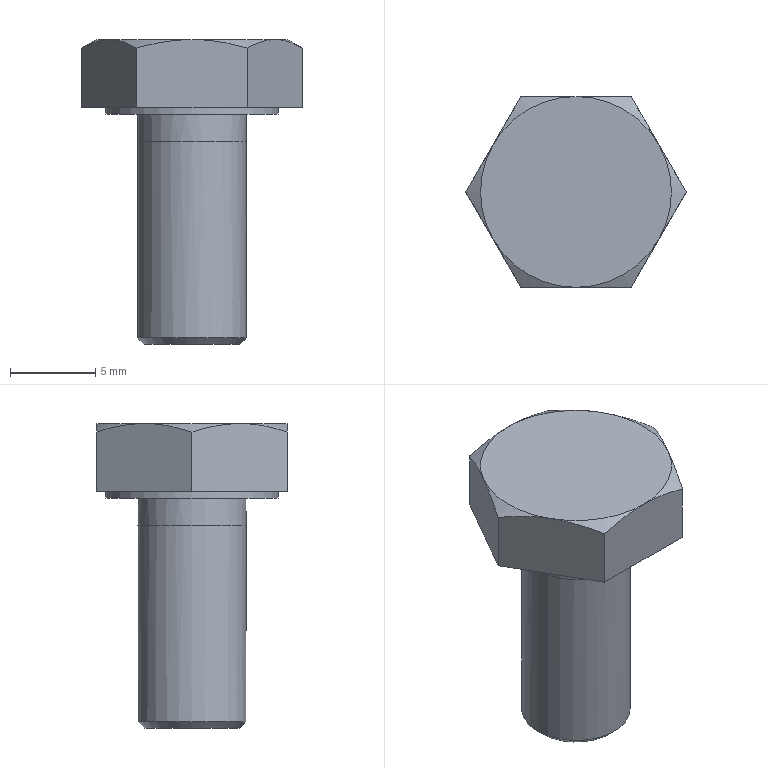Part | NX | features solid 2 | 1 solid | 20 faces | box 12.905 x 11.176 x 17.863 mm | volume 885.633 mm3 | plane 10 | cone 7 | cylinder 3 | commonest cylinder face diameters 6.35 x2 10.109 x1
STEP:
#1=CARTESIAN_POINT('',(-3.175,0.,-4.369));
#2=VERTEX_POINT('',#1);
#3=CARTESIAN_POINT('',(0.,0.,-4.369));
#4=DIRECTION('',(0.,0.,-1.));
#5=DIRECTION('',(-1.,0.,0.));
#6=AXIS2_PLACEMENT_3D('',#3,#4,#5);
#7=CIRCLE('',#6,3.175);
#8=EDGE_CURVE('',#2,#2,#7,.T.);
#9=ORIENTED_EDGE('',*,*,#8,.T.);
#10=EDGE_LOOP('',(#9));
#11=FACE_BOUND('',#10,.T.);
#12=CARTESIAN_POINT('',(-3.175,0.,-5.956));
#13=VERTEX_POINT('',#12);
#14=CARTESIAN_POINT('',(-2.488,2.488,-5.956));
#15=CARTESIAN_POINT('',(-3.519,0.,-5.956));
#16=CARTESIAN_POINT('',(-2.488,-2.488,-5.956));
#17=CARTESIAN_POINT('',(0.,-3.519,-5.956));
#18=CARTESIAN_POINT('',(2.488,-2.488,-5.956));
#19=CARTESIAN_POINT('',(3.519,0.,-5.956));
#20=CARTESIAN_POINT('',(2.488,2.488,-5.956));
#21=CARTESIAN_POINT('',(0.,3.519,-5.956));
#22=CARTESIAN_POINT('',(-2.488,2.488,-5.956));
#23=CARTESIAN_POINT('',(-3.519,0.,-5.956));
#24=CARTESIAN_POINT('',(-2.488,-2.488,-5.956));
#25=B_SPLINE_CURVE_WITH_KNOTS('',3,(#14,#15,#16,#17,#18,#19,#20,#21,#22,#23,#24),.UNSPECIFIED.,.T.,.F.,(1,1,1,1,1,1,1,1,1,1,1,1,1,1,1),(-0.375,-0.25,-0.125,0.,0.125,0.25,0.375,0.5,0.625,0.75,0.875,1.,1.125,1.25,1.375),.UNSPECIFIED.);
#26=EDGE_CURVE('',#13,#13,#25,.T.);
#27=ORIENTED_EDGE('',*,*,#26,.T.);
#28=EDGE_LOOP('',(#27));
#29=FACE_BOUND('',#28,.T.);
#30=CARTESIAN_POINT('',(0.,0.,0.));
#31=DIRECTION('',(0.,0.,-1.));
#32=DIRECTION('',(-1.,0.,0.));
#33=AXIS2_PLACEMENT_3D('',#30,#31,#32);
#34=CYLINDRICAL_SURFACE('',#33,3.175);
#35=ADVANCED_FACE('',(#11,#29),#34,.T.);
#36=CARTESIAN_POINT('',(-6.452,0.,-3.962));
#37=VERTEX_POINT('',#36);
#38=CARTESIAN_POINT('',(-3.226,5.588,-3.962));
#39=VERTEX_POINT('',#38);
#40=CARTESIAN_POINT('',(-3.576,4.983,-3.962));
#41=DIRECTION('',(0.5,0.866,0.));
#42=VECTOR('',#41,1000.);
#43=LINE('',#40,#42);
#44=EDGE_CURVE('',#37,#39,#43,.T.);
#45=ORIENTED_EDGE('',*,*,#44,.T.);
#46=CARTESIAN_POINT('',(3.226,5.588,-3.962));
#47=VERTEX_POINT('',#46);
#48=CARTESIAN_POINT('',(5.055,5.588,-3.962));
#49=DIRECTION('',(1.,0.,0.));
#50=VECTOR('',#49,1000.);
#51=LINE('',#48,#50);
#52=EDGE_CURVE('',#39,#47,#51,.T.);
#53=ORIENTED_EDGE('',*,*,#52,.T.);
#54=CARTESIAN_POINT('',(6.452,0.,-3.962));
#55=VERTEX_POINT('',#54);
#56=CARTESIAN_POINT('',(6.103,0.6053,-3.962));
#57=DIRECTION('',(0.5,-0.866,0.));
#58=VECTOR('',#57,1000.);
#59=LINE('',#56,#58);
#60=EDGE_CURVE('',#47,#55,#59,.T.);
#61=ORIENTED_EDGE('',*,*,#60,.T.);
#62=CARTESIAN_POINT('',(3.226,-5.588,-3.962));
#63=VERTEX_POINT('',#62);
#64=CARTESIAN_POINT('',(6.103,-0.6053,-3.962));
#65=DIRECTION('',(-0.5,-0.866,0.));
#66=VECTOR('',#65,1000.);
#67=LINE('',#64,#66);
#68=EDGE_CURVE('',#55,#63,#67,.T.);
#69=ORIENTED_EDGE('',*,*,#68,.T.);
#70=CARTESIAN_POINT('',(-3.226,-5.588,-3.962));
#71=VERTEX_POINT('',#70);
#72=CARTESIAN_POINT('',(5.055,-5.588,-3.962));
#73=DIRECTION('',(-1.,0.,0.));
#74=VECTOR('',#73,1000.);
#75=LINE('',#72,#74);
#76=EDGE_CURVE('',#63,#71,#75,.T.);
#77=ORIENTED_EDGE('',*,*,#76,.T.);
#78=CARTESIAN_POINT('',(-3.576,-4.983,-3.962));
#79=DIRECTION('',(-0.5,0.866,0.));
#80=VECTOR('',#79,1000.);
#81=LINE('',#78,#80);
#82=EDGE_CURVE('',#71,#37,#81,.T.);
#83=ORIENTED_EDGE('',*,*,#82,.T.);
#84=EDGE_LOOP('',(#45,#53,#61,#69,#77,#83));
#85=FACE_BOUND('',#84,.T.);
#86=CARTESIAN_POINT('',(-5.055,0.,-3.962));
#87=VERTEX_POINT('',#86);
#88=CARTESIAN_POINT('',(0.,0.,-3.962));
#89=DIRECTION('',(0.,0.,-1.));
#90=DIRECTION('',(-1.,0.,0.));
#91=AXIS2_PLACEMENT_3D('',#88,#89,#90);
#92=CIRCLE('',#91,5.055);
#93=EDGE_CURVE('',#87,#87,#92,.T.);
#94=ORIENTED_EDGE('',*,*,#93,.F.);
#95=EDGE_LOOP('',(#94));
#96=FACE_BOUND('',#95,.T.);
#97=CARTESIAN_POINT('',(5.055,0.,-3.962));
#98=DIRECTION('',(0.,0.,-1.));
#99=DIRECTION('',(-1.,0.,0.));
#100=AXIS2_PLACEMENT_3D('',#97,#98,#99);
#101=PLANE('',#100);
#102=ADVANCED_FACE('',(#85,#96),#101,.T.);
#103=CARTESIAN_POINT('',(-2.794,0.,-17.863));
#104=VERTEX_POINT('',#103);
#105=CARTESIAN_POINT('',(0.,0.,-17.863));
#106=DIRECTION('',(0.,0.,-1.));
#107=DIRECTION('',(-1.,0.,0.));
#108=AXIS2_PLACEMENT_3D('',#105,#106,#107);
#109=CIRCLE('',#108,2.794);
#110=EDGE_CURVE('',#104,#104,#109,.T.);
#111=ORIENTED_EDGE('',*,*,#110,.T.);
#112=EDGE_LOOP('',(#111));
#113=FACE_BOUND('',#112,.T.);
#114=CARTESIAN_POINT('',(0.,0.,-17.863));
#115=DIRECTION('',(0.,0.,-1.));
#116=DIRECTION('',(-1.,0.,0.));
#117=AXIS2_PLACEMENT_3D('',#114,#115,#116);
#118=PLANE('',#117);
#119=ADVANCED_FACE('',(#113),#118,.T.);
#120=CARTESIAN_POINT('',(-3.175,0.,-17.482));
#121=VERTEX_POINT('',#120);
#122=CARTESIAN_POINT('',(0.,0.,-17.482));
#123=DIRECTION('',(0.,0.,-1.));
#124=DIRECTION('',(-1.,0.,0.));
#125=AXIS2_PLACEMENT_3D('',#122,#123,#124);
#126=CIRCLE('',#125,3.175);
#127=EDGE_CURVE('',#121,#121,#126,.T.);
#128=ORIENTED_EDGE('',*,*,#127,.T.);
#129=EDGE_LOOP('',(#128));
#130=FACE_BOUND('',#129,.T.);
#131=ORIENTED_EDGE('',*,*,#110,.F.);
#132=EDGE_LOOP('',(#131));
#133=FACE_BOUND('',#132,.T.);
#134=CARTESIAN_POINT('',(0.,0.,-17.863));
#135=DIRECTION('',(0.,0.,1.));
#136=DIRECTION('',(1.,0.,0.));
#137=AXIS2_PLACEMENT_3D('',#134,#135,#136);
#138=CONICAL_SURFACE('',#137,2.794,0.7854);
#139=ADVANCED_FACE('',(#130,#133),#138,.T.);
#140=ORIENTED_EDGE('',*,*,#26,.F.);
#141=EDGE_LOOP('',(#140));
#142=FACE_BOUND('',#141,.T.);
#143=ORIENTED_EDGE('',*,*,#127,.F.);
#144=EDGE_LOOP('',(#143));
#145=FACE_BOUND('',#144,.T.);
#146=CARTESIAN_POINT('',(0.,0.,0.));
#147=DIRECTION('',(0.,0.,-1.));
#148=DIRECTION('',(-1.,0.,0.));
#149=AXIS2_PLACEMENT_3D('',#146,#147,#148);
#150=CYLINDRICAL_SURFACE('',#149,3.175);
#151=ADVANCED_FACE('',(#142,#145),#150,.T.);
#152=CARTESIAN_POINT('',(-5.055,0.,-4.369));
#153=VERTEX_POINT('',#152);
#154=CARTESIAN_POINT('',(0.,0.,-4.369));
#155=DIRECTION('',(0.,0.,-1.));
#156=DIRECTION('',(-1.,0.,0.));
#157=AXIS2_PLACEMENT_3D('',#154,#155,#156);
#158=CIRCLE('',#157,5.055);
#159=EDGE_CURVE('',#153,#153,#158,.T.);
#160=ORIENTED_EDGE('',*,*,#159,.T.);
#161=EDGE_LOOP('',(#160));
#162=FACE_BOUND('',#161,.T.);
#163=ORIENTED_EDGE('',*,*,#8,.F.);
#164=EDGE_LOOP('',(#163));
#165=FACE_BOUND('',#164,.T.);
#166=CARTESIAN_POINT('',(3.175,0.,-4.369));
#167=DIRECTION('',(0.,0.,-1.));
#168=DIRECTION('',(-1.,0.,0.));
#169=AXIS2_PLACEMENT_3D('',#166,#167,#168);
#170=PLANE('',#169);
#171=ADVANCED_FACE('',(#162,#165),#170,.T.);
#172=ORIENTED_EDGE('',*,*,#93,.T.);
#173=EDGE_LOOP('',(#172));
#174=FACE_BOUND('',#173,.T.);
#175=ORIENTED_EDGE('',*,*,#159,.F.);
#176=EDGE_LOOP('',(#175));
#177=FACE_BOUND('',#176,.T.);
#178=CARTESIAN_POINT('',(0.,0.,0.));
#179=DIRECTION('',(0.,0.,-1.));
#180=DIRECTION('',(-1.,0.,0.));
#181=AXIS2_PLACEMENT_3D('',#178,#179,#180);
#182=CYLINDRICAL_SURFACE('',#181,5.055);
#183=ADVANCED_FACE('',(#174,#177),#182,.T.);
#184=ORIENTED_EDGE('',*,*,#52,.F.);
#185=CARTESIAN_POINT('',(-3.226,5.588,-0.4991));
#186=VERTEX_POINT('',#185);
#187=CARTESIAN_POINT('',(-3.226,5.588,-19.649));
#188=DIRECTION('',(0.,0.,1.));
#189=VECTOR('',#188,1000.);
#190=LINE('',#187,#189);
#191=EDGE_CURVE('',#39,#186,#190,.T.);
#192=ORIENTED_EDGE('',*,*,#191,.T.);
#193=CARTESIAN_POINT('',(0.,5.588,0.));
#194=VERTEX_POINT('',#193);
#195=CARTESIAN_POINT('',(-3.226,5.588,-0.4991));
#196=CARTESIAN_POINT('',(-2.177,5.588,-0.1961));
#197=CARTESIAN_POINT('',(-1.09,5.588,0.));
#198=CARTESIAN_POINT('',(0.,5.588,0.));
#199=B_SPLINE_CURVE_WITH_KNOTS('',3,(#195,#196,#197,#198),.UNSPECIFIED.,.F.,.F.,(4,4),(0.005758,0.009022),.UNSPECIFIED.);
#200=EDGE_CURVE('',#194,#186,#199,.F.);
#201=ORIENTED_EDGE('',*,*,#200,.F.);
#202=CARTESIAN_POINT('',(3.226,5.588,-0.4991));
#203=VERTEX_POINT('',#202);
#204=CARTESIAN_POINT('',(0.,5.588,0.));
#205=CARTESIAN_POINT('',(1.091,5.588,0.));
#206=CARTESIAN_POINT('',(2.183,5.588,-0.1979));
#207=CARTESIAN_POINT('',(3.226,5.588,-0.4991));
#208=B_SPLINE_CURVE_WITH_KNOTS('',3,(#204,#205,#206,#207),.UNSPECIFIED.,.F.,.F.,(4,4),(0.009022,0.01229),.UNSPECIFIED.);
#209=EDGE_CURVE('',#203,#194,#208,.F.);
#210=ORIENTED_EDGE('',*,*,#209,.F.);
#211=CARTESIAN_POINT('',(3.226,5.588,-19.649));
#212=DIRECTION('',(0.,0.,1.));
#213=VECTOR('',#212,1000.);
#214=LINE('',#211,#213);
#215=EDGE_CURVE('',#47,#203,#214,.T.);
#216=ORIENTED_EDGE('',*,*,#215,.F.);
#217=EDGE_LOOP('',(#184,#192,#201,#210,#216));
#218=FACE_BOUND('',#217,.T.);
#219=CARTESIAN_POINT('',(3.226,5.588,-19.649));
#220=DIRECTION('',(0.,1.,0.));
#221=DIRECTION('',(0.,0.,1.));
#222=AXIS2_PLACEMENT_3D('',#219,#220,#221);
#223=PLANE('',#222);
#224=ADVANCED_FACE('',(#218),#223,.T.);
#225=ORIENTED_EDGE('',*,*,#44,.F.);
#226=CARTESIAN_POINT('',(-6.452,0.,-0.4991));
#227=VERTEX_POINT('',#226);
#228=CARTESIAN_POINT('',(-6.452,0.,-19.649));
#229=DIRECTION('',(0.,0.,1.));
#230=VECTOR('',#229,1000.);
#231=LINE('',#228,#230);
#232=EDGE_CURVE('',#37,#227,#231,.T.);
#233=ORIENTED_EDGE('',*,*,#232,.T.);
#234=CARTESIAN_POINT('',(-4.839,2.794,0.));
#235=VERTEX_POINT('',#234);
#236=CARTESIAN_POINT('',(-4.839,2.794,0.));
#237=CARTESIAN_POINT('',(-5.387,1.846,0.));
#238=CARTESIAN_POINT('',(-5.926,0.9118,-0.1952));
#239=CARTESIAN_POINT('',(-6.452,0.,-0.4991));
#240=B_SPLINE_CURVE_WITH_KNOTS('',3,(#236,#237,#238,#239),.UNSPECIFIED.,.F.,.F.,(4,4),(0.003265,0.006517),.UNSPECIFIED.);
#241=EDGE_CURVE('',#235,#227,#240,.T.);
#242=ORIENTED_EDGE('',*,*,#241,.F.);
#243=CARTESIAN_POINT('',(-3.226,5.588,-0.4991));
#244=CARTESIAN_POINT('',(-3.754,4.674,-0.1944));
#245=CARTESIAN_POINT('',(-4.29,3.746,0.));
#246=CARTESIAN_POINT('',(-4.839,2.794,0.));
#247=B_SPLINE_CURVE_WITH_KNOTS('',3,(#243,#244,#245,#246),.UNSPECIFIED.,.F.,.F.,(4,4),(0.000000238,0.003265),.UNSPECIFIED.);
#248=EDGE_CURVE('',#186,#235,#247,.T.);
#249=ORIENTED_EDGE('',*,*,#248,.F.);
#250=ORIENTED_EDGE('',*,*,#191,.F.);
#251=EDGE_LOOP('',(#225,#233,#242,#249,#250));
#252=FACE_BOUND('',#251,.T.);
#253=CARTESIAN_POINT('',(-3.226,5.588,-19.649));
#254=DIRECTION('',(-0.866,0.5,0.));
#255=DIRECTION('',(-0.5,-0.866,0.));
#256=AXIS2_PLACEMENT_3D('',#253,#254,#255);
#257=PLANE('',#256);
#258=ADVANCED_FACE('',(#252),#257,.T.);
#259=ORIENTED_EDGE('',*,*,#82,.F.);
#260=CARTESIAN_POINT('',(-3.226,-5.588,-0.4991));
#261=VERTEX_POINT('',#260);
#262=CARTESIAN_POINT('',(-3.226,-5.588,-19.649));
#263=DIRECTION('',(0.,0.,1.));
#264=VECTOR('',#263,1000.);
#265=LINE('',#262,#264);
#266=EDGE_CURVE('',#71,#261,#265,.T.);
#267=ORIENTED_EDGE('',*,*,#266,.T.);
#268=CARTESIAN_POINT('',(-4.839,-2.794,0.));
#269=VERTEX_POINT('',#268);
#270=CARTESIAN_POINT('',(-4.839,-2.794,0.));
#271=CARTESIAN_POINT('',(-4.292,-3.742,0.));
#272=CARTESIAN_POINT('',(-3.753,-4.676,-0.1952));
#273=CARTESIAN_POINT('',(-3.226,-5.588,-0.4991));
#274=B_SPLINE_CURVE_WITH_KNOTS('',3,(#270,#271,#272,#273),.UNSPECIFIED.,.F.,.F.,(4,4),(0.003265,0.006517),.UNSPECIFIED.);
#275=EDGE_CURVE('',#269,#261,#274,.T.);
#276=ORIENTED_EDGE('',*,*,#275,.F.);
#277=CARTESIAN_POINT('',(-6.452,0.,-0.4991));
#278=CARTESIAN_POINT('',(-5.925,-0.9141,-0.1944));
#279=CARTESIAN_POINT('',(-5.389,-1.842,0.));
#280=CARTESIAN_POINT('',(-4.839,-2.794,0.));
#281=B_SPLINE_CURVE_WITH_KNOTS('',3,(#277,#278,#279,#280),.UNSPECIFIED.,.F.,.F.,(4,4),(0.000000238,0.003265),.UNSPECIFIED.);
#282=EDGE_CURVE('',#227,#269,#281,.T.);
#283=ORIENTED_EDGE('',*,*,#282,.F.);
#284=ORIENTED_EDGE('',*,*,#232,.F.);
#285=EDGE_LOOP('',(#259,#267,#276,#283,#284));
#286=FACE_BOUND('',#285,.T.);
#287=CARTESIAN_POINT('',(-6.452,0.,-19.649));
#288=DIRECTION('',(-0.866,-0.5,0.));
#289=DIRECTION('',(0.5,-0.866,0.));
#290=AXIS2_PLACEMENT_3D('',#287,#288,#289);
#291=PLANE('',#290);
#292=ADVANCED_FACE('',(#286),#291,.T.);
#293=ORIENTED_EDGE('',*,*,#76,.F.);
#294=CARTESIAN_POINT('',(3.226,-5.588,-0.4991));
#295=VERTEX_POINT('',#294);
#296=CARTESIAN_POINT('',(3.226,-5.588,-19.649));
#297=DIRECTION('',(0.,0.,1.));
#298=VECTOR('',#297,1000.);
#299=LINE('',#296,#298);
#300=EDGE_CURVE('',#63,#295,#299,.T.);
#301=ORIENTED_EDGE('',*,*,#300,.T.);
#302=CARTESIAN_POINT('',(0.,-5.588,0.));
#303=VERTEX_POINT('',#302);
#304=CARTESIAN_POINT('',(0.,-5.588,0.));
#305=CARTESIAN_POINT('',(1.091,-5.588,0.));
#306=CARTESIAN_POINT('',(2.183,-5.588,-0.1979));
#307=CARTESIAN_POINT('',(3.226,-5.588,-0.4991));
#308=B_SPLINE_CURVE_WITH_KNOTS('',3,(#304,#305,#306,#307),.UNSPECIFIED.,.F.,.F.,(4,4),(0.009022,0.01229),.UNSPECIFIED.);
#309=EDGE_CURVE('',#303,#295,#308,.T.);
#310=ORIENTED_EDGE('',*,*,#309,.F.);
#311=CARTESIAN_POINT('',(-3.226,-5.588,-0.4991));
#312=CARTESIAN_POINT('',(-2.177,-5.588,-0.1961));
#313=CARTESIAN_POINT('',(-1.09,-5.588,0.));
#314=CARTESIAN_POINT('',(0.,-5.588,0.));
#315=B_SPLINE_CURVE_WITH_KNOTS('',3,(#311,#312,#313,#314),.UNSPECIFIED.,.F.,.F.,(4,4),(0.005758,0.009022),.UNSPECIFIED.);
#316=EDGE_CURVE('',#261,#303,#315,.T.);
#317=ORIENTED_EDGE('',*,*,#316,.F.);
#318=ORIENTED_EDGE('',*,*,#266,.F.);
#319=EDGE_LOOP('',(#293,#301,#310,#317,#318));
#320=FACE_BOUND('',#319,.T.);
#321=CARTESIAN_POINT('',(-3.226,-5.588,-19.649));
#322=DIRECTION('',(0.,-1.,0.));
#323=DIRECTION('',(0.,0.,-1.));
#324=AXIS2_PLACEMENT_3D('',#321,#322,#323);
#325=PLANE('',#324);
#326=ADVANCED_FACE('',(#320),#325,.T.);
#327=ORIENTED_EDGE('',*,*,#68,.F.);
#328=CARTESIAN_POINT('',(6.452,0.,-0.4991));
#329=VERTEX_POINT('',#328);
#330=CARTESIAN_POINT('',(6.452,0.,-19.649));
#331=DIRECTION('',(0.,0.,1.));
#332=VECTOR('',#331,1000.);
#333=LINE('',#330,#332);
#334=EDGE_CURVE('',#55,#329,#333,.T.);
#335=ORIENTED_EDGE('',*,*,#334,.T.);
#336=CARTESIAN_POINT('',(4.839,-2.794,0.));
#337=VERTEX_POINT('',#336);
#338=CARTESIAN_POINT('',(4.839,-2.794,0.));
#339=CARTESIAN_POINT('',(5.387,-1.846,0.));
#340=CARTESIAN_POINT('',(5.926,-0.9118,-0.1952));
#341=CARTESIAN_POINT('',(6.452,0.,-0.4991));
#342=B_SPLINE_CURVE_WITH_KNOTS('',3,(#338,#339,#340,#341),.UNSPECIFIED.,.F.,.F.,(4,4),(0.003265,0.006517),.UNSPECIFIED.);
#343=EDGE_CURVE('',#337,#329,#342,.T.);
#344=ORIENTED_EDGE('',*,*,#343,.F.);
#345=CARTESIAN_POINT('',(3.226,-5.588,-0.4991));
#346=CARTESIAN_POINT('',(3.754,-4.674,-0.1944));
#347=CARTESIAN_POINT('',(4.29,-3.746,0.));
#348=CARTESIAN_POINT('',(4.839,-2.794,0.));
#349=B_SPLINE_CURVE_WITH_KNOTS('',3,(#345,#346,#347,#348),.UNSPECIFIED.,.F.,.F.,(4,4),(0.000000238,0.003265),.UNSPECIFIED.);
#350=EDGE_CURVE('',#295,#337,#349,.T.);
#351=ORIENTED_EDGE('',*,*,#350,.F.);
#352=ORIENTED_EDGE('',*,*,#300,.F.);
#353=EDGE_LOOP('',(#327,#335,#344,#351,#352));
#354=FACE_BOUND('',#353,.T.);
#355=CARTESIAN_POINT('',(3.226,-5.588,-19.649));
#356=DIRECTION('',(0.866,-0.5,0.));
#357=DIRECTION('',(0.5,0.866,0.));
#358=AXIS2_PLACEMENT_3D('',#355,#356,#357);
#359=PLANE('',#358);
#360=ADVANCED_FACE('',(#354),#359,.T.);
#361=ORIENTED_EDGE('',*,*,#60,.F.);
#362=ORIENTED_EDGE('',*,*,#215,.T.);
#363=CARTESIAN_POINT('',(4.839,2.794,0.));
#364=VERTEX_POINT('',#363);
#365=CARTESIAN_POINT('',(4.839,2.794,0.));
#366=CARTESIAN_POINT('',(4.292,3.742,0.));
#367=CARTESIAN_POINT('',(3.753,4.676,-0.1952));
#368=CARTESIAN_POINT('',(3.226,5.588,-0.4991));
#369=B_SPLINE_CURVE_WITH_KNOTS('',3,(#365,#366,#367,#368),.UNSPECIFIED.,.F.,.F.,(4,4),(0.003265,0.006517),.UNSPECIFIED.);
#370=EDGE_CURVE('',#364,#203,#369,.T.);
#371=ORIENTED_EDGE('',*,*,#370,.F.);
#372=CARTESIAN_POINT('',(6.452,0.,-0.4991));
#373=CARTESIAN_POINT('',(5.925,0.9141,-0.1944));
#374=CARTESIAN_POINT('',(5.389,1.842,0.));
#375=CARTESIAN_POINT('',(4.839,2.794,0.));
#376=B_SPLINE_CURVE_WITH_KNOTS('',3,(#372,#373,#374,#375),.UNSPECIFIED.,.F.,.F.,(4,4),(0.000000238,0.003265),.UNSPECIFIED.);
#377=EDGE_CURVE('',#329,#364,#376,.T.);
#378=ORIENTED_EDGE('',*,*,#377,.F.);
#379=ORIENTED_EDGE('',*,*,#334,.F.);
#380=EDGE_LOOP('',(#361,#362,#371,#378,#379));
#381=FACE_BOUND('',#380,.T.);
#382=CARTESIAN_POINT('',(6.452,0.,-19.649));
#383=DIRECTION('',(0.866,0.5,0.));
#384=DIRECTION('',(-0.5,0.866,0.));
#385=AXIS2_PLACEMENT_3D('',#382,#383,#384);
#386=PLANE('',#385);
#387=ADVANCED_FACE('',(#381),#386,.T.);
#388=CARTESIAN_POINT('',(0.,0.,0.));
#389=DIRECTION('',(0.,0.,-1.));
#390=DIRECTION('',(-1.,0.,0.));
#391=AXIS2_PLACEMENT_3D('',#388,#389,#390);
#392=CIRCLE('',#391,5.588);
#393=EDGE_CURVE('',#364,#337,#392,.T.);
#394=ORIENTED_EDGE('',*,*,#393,.T.);
#395=ORIENTED_EDGE('',*,*,#343,.T.);
#396=ORIENTED_EDGE('',*,*,#377,.T.);
#397=EDGE_LOOP('',(#394,#395,#396));
#398=FACE_BOUND('',#397,.T.);
#399=CARTESIAN_POINT('',(0.,0.,-0.5133));
#400=DIRECTION('',(0.,0.,-1.));
#401=DIRECTION('',(-1.,0.,0.));
#402=AXIS2_PLACEMENT_3D('',#399,#400,#401);
#403=CONICAL_SURFACE('',#402,6.477,1.047);
#404=ADVANCED_FACE('',(#398),#403,.T.);
#405=CARTESIAN_POINT('',(0.,0.,0.));
#406=DIRECTION('',(0.,0.,-1.));
#407=DIRECTION('',(-1.,0.,0.));
#408=AXIS2_PLACEMENT_3D('',#405,#406,#407);
#409=CIRCLE('',#408,5.588);
#410=EDGE_CURVE('',#337,#303,#409,.T.);
#411=ORIENTED_EDGE('',*,*,#410,.T.);
#412=ORIENTED_EDGE('',*,*,#309,.T.);
#413=ORIENTED_EDGE('',*,*,#350,.T.);
#414=EDGE_LOOP('',(#411,#412,#413));
#415=FACE_BOUND('',#414,.T.);
#416=CARTESIAN_POINT('',(0.,0.,-0.5133));
#417=DIRECTION('',(0.,0.,-1.));
#418=DIRECTION('',(-1.,0.,0.));
#419=AXIS2_PLACEMENT_3D('',#416,#417,#418);
#420=CONICAL_SURFACE('',#419,6.477,1.047);
#421=ADVANCED_FACE('',(#415),#420,.T.);
#422=CARTESIAN_POINT('',(0.,0.,0.));
#423=DIRECTION('',(0.,0.,-1.));
#424=DIRECTION('',(-1.,0.,0.));
#425=AXIS2_PLACEMENT_3D('',#422,#423,#424);
#426=CIRCLE('',#425,5.588);
#427=EDGE_CURVE('',#303,#269,#426,.T.);
#428=ORIENTED_EDGE('',*,*,#427,.T.);
#429=ORIENTED_EDGE('',*,*,#275,.T.);
#430=ORIENTED_EDGE('',*,*,#316,.T.);
#431=EDGE_LOOP('',(#428,#429,#430));
#432=FACE_BOUND('',#431,.T.);
#433=CARTESIAN_POINT('',(0.,0.,-0.5133));
#434=DIRECTION('',(0.,0.,-1.));
#435=DIRECTION('',(-1.,0.,0.));
#436=AXIS2_PLACEMENT_3D('',#433,#434,#435);
#437=CONICAL_SURFACE('',#436,6.477,1.047);
#438=ADVANCED_FACE('',(#432),#437,.T.);
#439=CARTESIAN_POINT('',(0.,0.,0.));
#440=DIRECTION('',(0.,0.,-1.));
#441=DIRECTION('',(-1.,0.,0.));
#442=AXIS2_PLACEMENT_3D('',#439,#440,#441);
#443=CIRCLE('',#442,5.588);
#444=EDGE_CURVE('',#269,#235,#443,.T.);
#445=ORIENTED_EDGE('',*,*,#444,.T.);
#446=ORIENTED_EDGE('',*,*,#241,.T.);
#447=ORIENTED_EDGE('',*,*,#282,.T.);
#448=EDGE_LOOP('',(#445,#446,#447));
#449=FACE_BOUND('',#448,.T.);
#450=CARTESIAN_POINT('',(0.,0.,-0.5133));
#451=DIRECTION('',(0.,0.,-1.));
#452=DIRECTION('',(-1.,0.,0.));
#453=AXIS2_PLACEMENT_3D('',#450,#451,#452);
#454=CONICAL_SURFACE('',#453,6.477,1.047);
#455=ADVANCED_FACE('',(#449),#454,.T.);
#456=CARTESIAN_POINT('',(0.,0.,0.));
#457=DIRECTION('',(0.,0.,-1.));
#458=DIRECTION('',(-1.,0.,0.));
#459=AXIS2_PLACEMENT_3D('',#456,#457,#458);
#460=CIRCLE('',#459,5.588);
#461=EDGE_CURVE('',#235,#194,#460,.T.);
#462=ORIENTED_EDGE('',*,*,#461,.T.);
#463=ORIENTED_EDGE('',*,*,#200,.T.);
#464=ORIENTED_EDGE('',*,*,#248,.T.);
#465=EDGE_LOOP('',(#462,#463,#464));
#466=FACE_BOUND('',#465,.T.);
#467=CARTESIAN_POINT('',(0.,0.,-0.5133));
#468=DIRECTION('',(0.,0.,-1.));
#469=DIRECTION('',(-1.,0.,0.));
#470=AXIS2_PLACEMENT_3D('',#467,#468,#469);
#471=CONICAL_SURFACE('',#470,6.477,1.047);
#472=ADVANCED_FACE('',(#466),#471,.T.);
#473=ORIENTED_EDGE('',*,*,#461,.F.);
#474=ORIENTED_EDGE('',*,*,#444,.F.);
#475=ORIENTED_EDGE('',*,*,#427,.F.);
#476=ORIENTED_EDGE('',*,*,#410,.F.);
#477=ORIENTED_EDGE('',*,*,#393,.F.);
#478=CARTESIAN_POINT('',(0.,0.,0.));
#479=DIRECTION('',(0.,0.,-1.));
#480=DIRECTION('',(-1.,0.,0.));
#481=AXIS2_PLACEMENT_3D('',#478,#479,#480);
#482=CIRCLE('',#481,5.588);
#483=EDGE_CURVE('',#194,#364,#482,.T.);
#484=ORIENTED_EDGE('',*,*,#483,.F.);
#485=EDGE_LOOP('',(#473,#474,#475,#476,#477,#484));
#486=FACE_BOUND('',#485,.T.);
#487=CARTESIAN_POINT('',(5.588,0.,0.));
#488=DIRECTION('',(0.,0.,1.));
#489=DIRECTION('',(1.,0.,0.));
#490=AXIS2_PLACEMENT_3D('',#487,#488,#489);
#491=PLANE('',#490);
#492=ADVANCED_FACE('',(#486),#491,.T.);
#493=ORIENTED_EDGE('',*,*,#370,.T.);
#494=ORIENTED_EDGE('',*,*,#209,.T.);
#495=ORIENTED_EDGE('',*,*,#483,.T.);
#496=EDGE_LOOP('',(#493,#494,#495));
#497=FACE_BOUND('',#496,.T.);
#498=CARTESIAN_POINT('',(0.,0.,-0.5133));
#499=DIRECTION('',(0.,0.,-1.));
#500=DIRECTION('',(-1.,0.,0.));
#501=AXIS2_PLACEMENT_3D('',#498,#499,#500);
#502=CONICAL_SURFACE('',#501,6.477,1.047);
#503=ADVANCED_FACE('',(#497),#502,.T.);
#504=CLOSED_SHELL('',(#35,#102,#119,#139,#151,#171,#183,#224,#258,#292,#326,#360,#387,#404,#421,#438,#455,#472,#492,#503));
#505=MANIFOLD_SOLID_BREP('',#504);
#506=(LENGTH_UNIT()NAMED_UNIT(*)SI_UNIT(.MILLI.,.METRE.));
#507=UNCERTAINTY_MEASURE_WITH_UNIT(LENGTH_MEASURE(0.0508),#506,'','');
#508=(NAMED_UNIT(*)PLANE_ANGLE_UNIT()SI_UNIT($,.RADIAN.));
#509=(NAMED_UNIT(*)SI_UNIT($,.STERADIAN.)SOLID_ANGLE_UNIT());
#510=(GEOMETRIC_REPRESENTATION_CONTEXT(3)GLOBAL_UNCERTAINTY_ASSIGNED_CONTEXT((#507))GLOBAL_UNIT_ASSIGNED_CONTEXT((#506,#508,#509))REPRESENTATION_CONTEXT('',''));
#511=ADVANCED_BREP_SHAPE_REPRESENTATION('',(#505),#510);